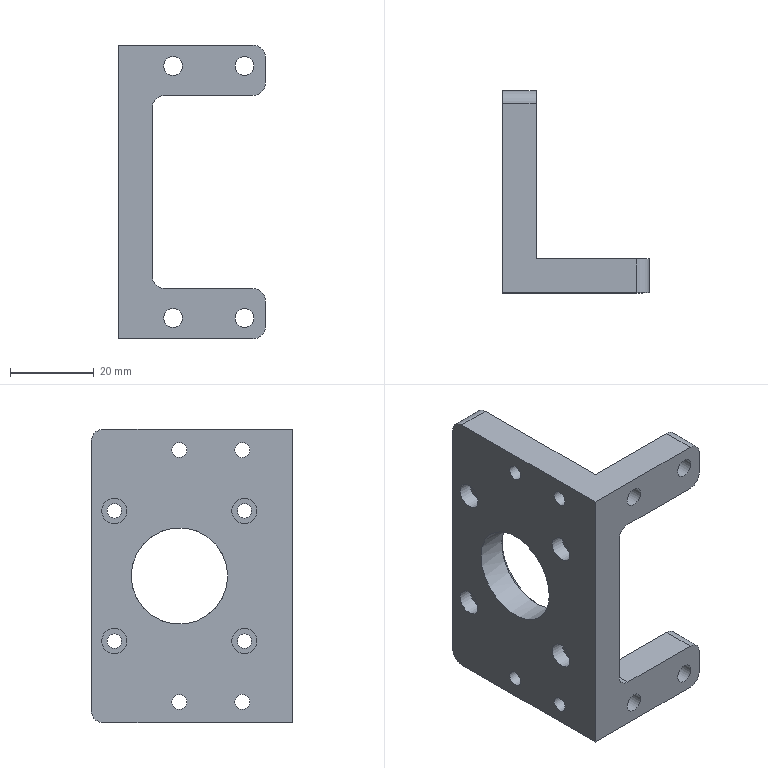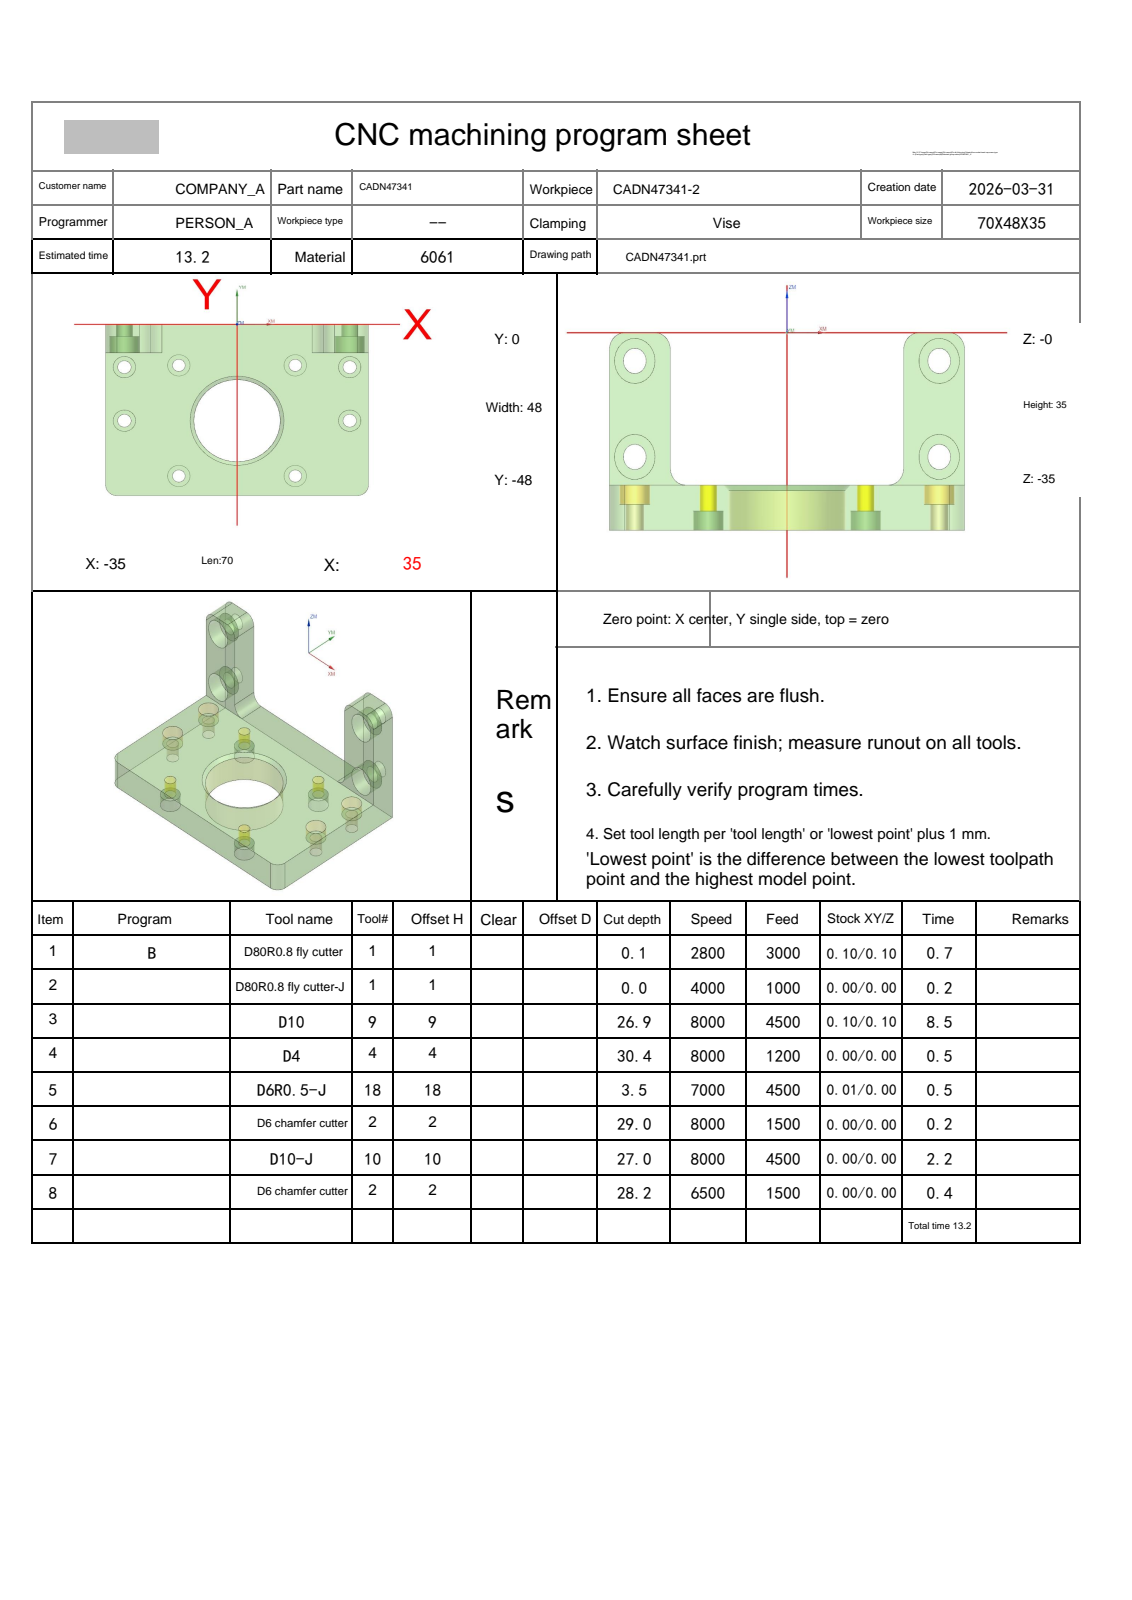NC program | NX | posted by the shop | part box 35 x 48 x 70 mm
Lines 1 to 110 of 13995:
%
O0001
(Machine time: 14.80 MIN)
(===Total Tool:6===)
(T1=D80R0.8 fly cutter D=80.  R=0.8  D-  H01 Z=0.    )
(T9=D10     D=10.  R=0.   D-  H09 Z=-26.9 )
(T4=D4      D=4.   R=0.   D-  H04 Z=-30.4 )
(T18=D6R0.5-J D=6.   R=0.5  D-  H18 Z=-3.5  )
(T2=D6 chamfer cutter   D=6.   R=0.   D-  H02 Z=-29.  )
(T10=D10-J  D=10.  R=0.   D10 H10 Z=-27.  )
G80 G90 G17 G49 G40
G91 G28 Z0
M01
N1 T01 M06
(D80R0.8 fly cutter  D=80. R=0.8 H=01 ce=0.10 di=0.10)
G00 G90 G54 X87.097 Y-24. M03 S2800
G43 H01 Z20.
M08
Z6.011
G01 Z4.011 F3000.
X75.097
X-75.097
X-87.097
Z6.011
G00 X87.097
Z5.522
G01 Z3.522
X75.097
X-75.097
X-87.097
Z5.522
G00 X87.097
Z5.033
G01 Z3.033
X75.097
X-75.097
X-87.097
Z5.033
G00 X87.097
Z4.544
G01 Z2.544
X75.097
X-75.097
X-87.097
Z4.544
G00 Z20.
X87.097
Z4.056
G01 Z2.056
X75.097
X-75.097
X-87.097
Z4.056
G00 Z20.
X87.097
Z3.567
G01 Z1.567
X75.097
X-75.097
X-87.097
Z3.567
G00 Z20.
X87.097
Z3.078
G01 Z1.078
X75.097
X-75.097
X-87.097
Z3.078
G00 Z20.
X87.097
Z2.589
G01 Z.589
X75.097
X-75.097
X-87.097
Z2.589
G00 Z20.
X87.097
Z2.1
G01 Z.1
X75.097
X-75.097
X-87.097
Z2.1
G00 Z20.
G91 G28 Z0.0
M05
M09
G91 G28 Z0.0
M01
N2 T01 M06
(D80R0.8 fly cutter-J  D=80. R=0.8 H=01 ce=0.00 di=0.00)
G00 G90 G54 X86.999 Y-23.998 M03 S4000
G43 H01 Z20.
M08
Z2.
G01 Z0.0 F1000.
X74.999
X-74.999 Y-24.002
X-86.999
Z2.
G00 Z20.
G91 G28 Z0.0
M05
M09
G91 G28 Z0.0
M01